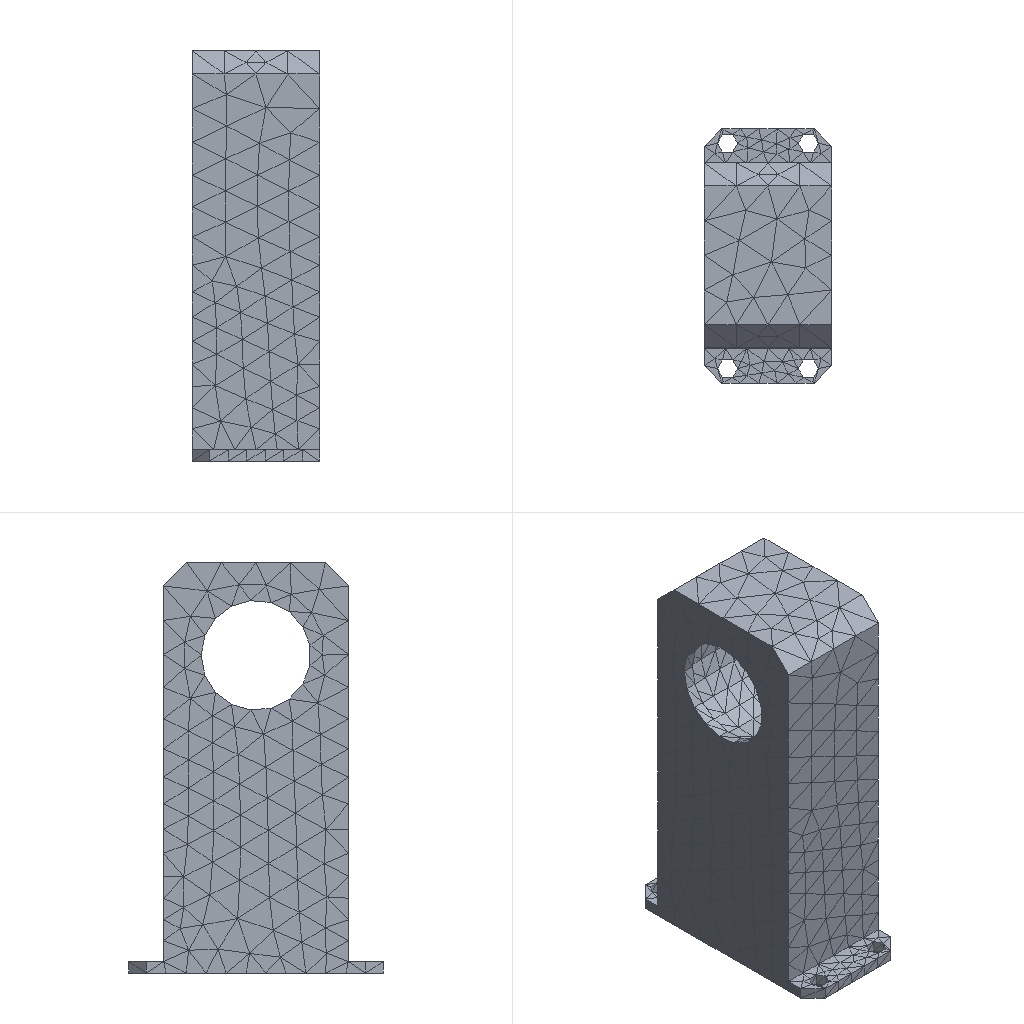Simulation study | nx simcenter
Set-up summary:
category,name,step,type,value,unit,region
solver,nx_nastran (Simcenter)
units,not stated in the deck,,not stated
analysis,deck,,static,static
analysis,solution,,SOL,101
load_step,SUBCASE 1,1,SUBCASE,SPC=1 LOAD=2
load_step,requested,,,1
mesh,nodes,,,4861
mesh,elements,,,2485
element_type,CTETRA,,solid,2485
load,nodal force total,,FX,0.0,model units
load,nodal force total,,FY,0.0,model units
load,nodal force total,,FZ,-1500000.06,model units
load,load commands in deck,,count,210
bc,support commands in deck,,count,481
analysis,NX solution 0,,Structural,Linear Statics - Single Constraint
check,setup vs results,,match,every grid point's frame and coordinates and every element id; grid points of CTETRA elements
Nastran input file, long lists of numbers shortened:
$*$$$$$$$$$$$$$$$$$$$$$$$$$$$$$$$$$$$$$$$$$$$$$$$$$$$$$$$$$$$$$$$$$
$*
$*                    NX v10.0.0.24 TRANSLATOR
$*                    FOR NX NASTRAN VERSION 10.0
$ (33 more lines like these left out)
ASSIGN OUTPUT2='146_sim1-solution_1.op2' UNIT=12
$*
$*$$$$$$$$$$$$$$$$$$$$$$$$$$$$$$$$$$$
$*
$* EXECUTIVE CONTROL
$*
$*$$$$$$$$$$$$$$$$$$$$$$$$$$$$$$$$$$$
$*
ID,NASTRAN,146_sim1-solution_1
SOL 101
CEND
$*
$*$$$$$$$$$$$$$$$$$$$$$$$$$$$$$$$$$$$
$*
$* CASE CONTROL
$*
$*$$$$$$$$$$$$$$$$$$$$$$$$$$$$$$$$$$$
$*
TITLE = Solution 1
ECHO = NONE
SPC = 1
OUTPUT
BCRESULTS(TRACTION,FORCE,PLOT) = ALL
DISPLACEMENT(PLOT) = ALL
ESE(PLOT) = ALL
FORCE(PLOT,CORNER) = ALL
OLOAD(PLOT) = ALL
SPCFORCES(PLOT) = ALL
STRAIN(PLOT,FIBER,CORNER) = ALL
STRESS(PLOT,CORNER) = ALL
$*  NX Step: Subcase - Static Loads 1
SUBCASE 1
LABEL = Subcase - Static Loads 1
LOAD = 2
$*
$*$$$$$$$$$$$$$$$$$$$$$$$$$$$$$$$$$$$
$*
$* BULK DATA
$*
$*$$$$$$$$$$$$$$$$$$$$$$$$$$$$$$$$$$$
$*
BEGIN BULK
$*
$* PARAM CARDS
$*
PARAM      K6ROT100.0000
PARAM     OIBULK     YES
PARAM    OMACHPR     YES
PARAM       POST      -2
PARAM    POSTEXT     YES
PARAM    UNITSYS   MN-MM
$*
$* GRID CARDS
$*
GRID*               4817               00.0000000000E+00-2.600000000E+01+
*       -5.600000000E+01               0
GRID*               4818               00.0000000000E+00-2.600000000E+01+
*       -5.400000000E+01               0
$ (9718 more lines like these left out)
$*
$* ELEMENT CARDS
$*
$*  NX Mesh Collector: Solid(1)
$*  NX Mesh: 3d_mesh(1)
CTETRA         1       1    2556       1    4369    2568      97      98+
+             99    2675     100     101
CTETRA         2       1       2       3    2557    2556     102     103+
+            104     105     106    2658
$ (4966 more lines like these left out)
$*
$* PROPERTY CARDS
$*
$*  NX Property: PSOLID1
PSOLID         1       2       0                           SMECH
$*
$* MATERIAL CARDS
$*
$*  NX Material: 6061
MAT1           27.3119+7        0.3300002.7500-62.1355-5
MATT1          2       1               2               3
TABLEM1        1                                                        +
+        20.00007.3119+7 21.11007.3119+7 23.89007.3119+7 37.78007.3119+7+
+        51.67007.3119+7 65.56007.2429+7 79.44007.2429+7 93.33007.1739+7+
+       107.22007.1049+7121.11007.0359+7135.00006.9670+7148.89006.8980+7+
+       162.78006.8290+7176.67006.6910+7190.56006.6221+7204.44006.4841+7+
+       218.33006.3461+7232.22006.1392+7246.11006.0012+7260.00005.8633+7+
+       273.89005.7253+7287.78005.5184+7301.67005.3804+7315.56005.1735+7+
+       329.44004.9665+7343.33004.7596+7357.22004.6216+7371.11004.4147+7+
+           ENDT
TABLEM1        2                                                        +
+        20.00000.330000 21.11000.330000    ENDT
TABLEM1        3                                                        +
+        20.00002.1600-5 93.33002.2500-5107.22002.2662-5121.11002.2824-5+
+       135.00002.2968-5148.89002.3130-5162.78002.3274-5176.67002.3418-5+
+       190.56002.3544-5204.44002.3688-5218.33002.3814-5232.22002.3958-5+
+       246.11002.4066-5260.00002.4192-5273.89002.4300-5287.78002.4408-5+
+       301.67002.4498-5315.56002.4606-5329.44002.4696-5343.33002.4786-5+
+       357.22002.4876-5371.11002.4984-5385.00002.5110-5398.89002.5254-5+
+       412.78002.5398-5426.67002.5560-5    ENDT
$*
$* LOAD AND CONSTRAINT CARDS
$*
$*  NX Load and Constraint: Fixed(1)
SPC            1    2527  123456  0.0000
SPC            1    2528  123456  0.0000
SPC            1    2529  123456  0.0000
SPC            1    2530  123456  0.0000
$ (477 more lines like these left out)
$*  NX Load and Constraint: Force(1)
FORCE          2    3687       0 7936.54  0.0000  0.0000-1.00000
FORCE          2    3688       0 7936.55  0.0000  0.0000-1.00000
FORCE          2    3689       0 7936.59  0.0000  0.0000-1.00000
FORCE          2    3690       0 7936.50  0.0000  0.0000-1.00000
$ (206 more lines like these left out)
ENDDATA 5c4b03b4
Results summary:
result,analysis,,,static
result,last_loadstep,,,1
result,primary field,,,displacements
result,reaction total,,FX,0.01097,model units
result,reaction total,,FY,0.02289,model units
result,reaction total,,FZ,1500000.125,model units
result,NX solution 0,,loadcases,1,mm